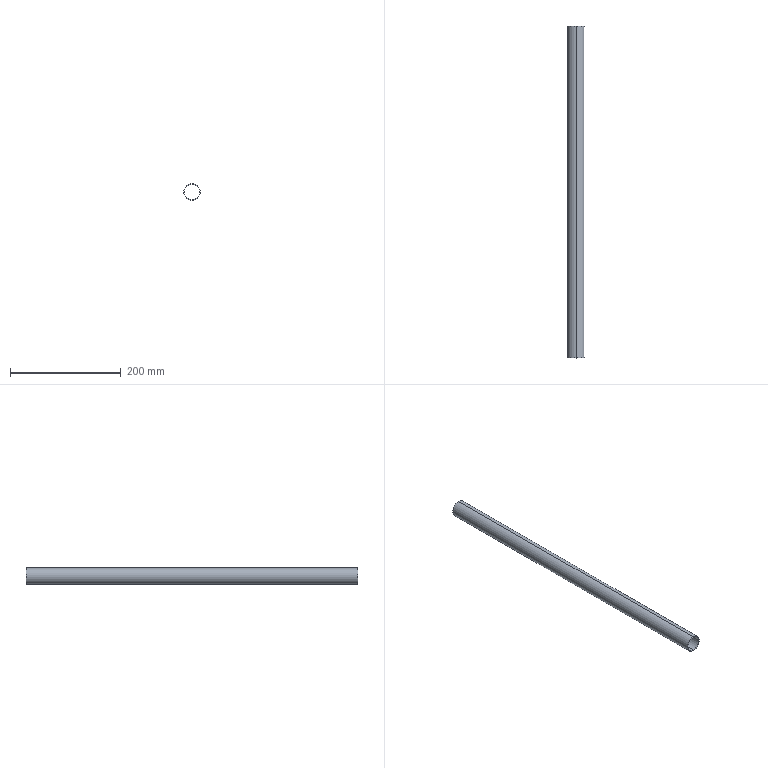Part | SolidWorks | features Sweep 1 | 1 solid | 6 faces | box 30 x 600 x 30 mm | volume 54664 mm3 | cylinder 4 | plane 2 | commonest cylinder face diameters 28 x2 30 x2
STEP:
#1=CARTESIAN_POINT('',(0.,0.,-14.));
#2=VERTEX_POINT('',#1);
#3=CARTESIAN_POINT('',(0.,0.,14.));
#4=VERTEX_POINT('',#3);
#5=CARTESIAN_POINT('',(0.,0.,0.));
#6=DIRECTION('',(0.,1.,0.));
#7=DIRECTION('',(0.,0.,1.));
#8=AXIS2_PLACEMENT_3D('',#5,#6,#7);
#9=CIRCLE('',#8,14.);
#10=EDGE_CURVE('',#2,#4,#9,.T.);
#11=ORIENTED_EDGE('',*,*,#10,.F.);
#12=CARTESIAN_POINT('',(0.,600.,-14.));
#13=VERTEX_POINT('',#12);
#14=CARTESIAN_POINT('',(0.,0.,-14.));
#15=DIRECTION('',(0.,1.,0.));
#16=VECTOR('',#15,1000.);
#17=LINE('',#14,#16);
#18=EDGE_CURVE('',#2,#13,#17,.T.);
#19=ORIENTED_EDGE('',*,*,#18,.T.);
#20=CARTESIAN_POINT('',(0.,600.,14.));
#21=VERTEX_POINT('',#20);
#22=CARTESIAN_POINT('',(0.,600.,0.));
#23=DIRECTION('',(0.,1.,0.));
#24=DIRECTION('',(0.,0.,1.));
#25=AXIS2_PLACEMENT_3D('',#22,#23,#24);
#26=CIRCLE('',#25,14.);
#27=EDGE_CURVE('',#13,#21,#26,.T.);
#28=ORIENTED_EDGE('',*,*,#27,.T.);
#29=CARTESIAN_POINT('',(0.,0.,14.));
#30=DIRECTION('',(0.,1.,0.));
#31=VECTOR('',#30,1000.);
#32=LINE('',#29,#31);
#33=EDGE_CURVE('',#4,#21,#32,.T.);
#34=ORIENTED_EDGE('',*,*,#33,.F.);
#35=EDGE_LOOP('',(#11,#19,#28,#34));
#36=FACE_OUTER_BOUND('',#35,.T.);
#37=CARTESIAN_POINT('',(0.,0.,0.));
#38=DIRECTION('',(0.,1.,0.));
#39=DIRECTION('',(0.,0.,1.));
#40=AXIS2_PLACEMENT_3D('',#37,#38,#39);
#41=CYLINDRICAL_SURFACE('',#40,14.);
#42=ADVANCED_FACE('',(#36),#41,.F.);
#43=CARTESIAN_POINT('',(0.,0.,15.));
#44=VERTEX_POINT('',#43);
#45=CARTESIAN_POINT('',(0.,0.,-15.));
#46=VERTEX_POINT('',#45);
#47=CARTESIAN_POINT('',(0.,0.,0.));
#48=DIRECTION('',(0.,1.,0.));
#49=DIRECTION('',(0.,0.,1.));
#50=AXIS2_PLACEMENT_3D('',#47,#48,#49);
#51=CIRCLE('',#50,15.);
#52=EDGE_CURVE('',#44,#46,#51,.T.);
#53=ORIENTED_EDGE('',*,*,#52,.T.);
#54=CARTESIAN_POINT('',(0.,600.,-15.));
#55=VERTEX_POINT('',#54);
#56=CARTESIAN_POINT('',(0.,0.,-15.));
#57=DIRECTION('',(0.,1.,0.));
#58=VECTOR('',#57,1000.);
#59=LINE('',#56,#58);
#60=EDGE_CURVE('',#46,#55,#59,.T.);
#61=ORIENTED_EDGE('',*,*,#60,.T.);
#62=CARTESIAN_POINT('',(0.,600.,15.));
#63=VERTEX_POINT('',#62);
#64=CARTESIAN_POINT('',(0.,600.,0.));
#65=DIRECTION('',(0.,1.,0.));
#66=DIRECTION('',(0.,0.,1.));
#67=AXIS2_PLACEMENT_3D('',#64,#65,#66);
#68=CIRCLE('',#67,15.);
#69=EDGE_CURVE('',#63,#55,#68,.T.);
#70=ORIENTED_EDGE('',*,*,#69,.F.);
#71=CARTESIAN_POINT('',(0.,0.,15.));
#72=DIRECTION('',(0.,1.,0.));
#73=VECTOR('',#72,1000.);
#74=LINE('',#71,#73);
#75=EDGE_CURVE('',#44,#63,#74,.T.);
#76=ORIENTED_EDGE('',*,*,#75,.F.);
#77=EDGE_LOOP('',(#53,#61,#70,#76));
#78=FACE_OUTER_BOUND('',#77,.T.);
#79=CARTESIAN_POINT('',(0.,0.,0.));
#80=DIRECTION('',(0.,1.,0.));
#81=DIRECTION('',(0.,0.,1.));
#82=AXIS2_PLACEMENT_3D('',#79,#80,#81);
#83=CYLINDRICAL_SURFACE('',#82,15.);
#84=ADVANCED_FACE('',(#78),#83,.T.);
#85=ORIENTED_EDGE('',*,*,#60,.F.);
#86=CARTESIAN_POINT('',(0.,0.,0.));
#87=DIRECTION('',(0.,1.,0.));
#88=DIRECTION('',(0.,0.,1.));
#89=AXIS2_PLACEMENT_3D('',#86,#87,#88);
#90=CIRCLE('',#89,15.);
#91=EDGE_CURVE('',#46,#44,#90,.T.);
#92=ORIENTED_EDGE('',*,*,#91,.T.);
#93=ORIENTED_EDGE('',*,*,#75,.T.);
#94=CARTESIAN_POINT('',(0.,600.,0.));
#95=DIRECTION('',(0.,1.,0.));
#96=DIRECTION('',(0.,0.,1.));
#97=AXIS2_PLACEMENT_3D('',#94,#95,#96);
#98=CIRCLE('',#97,15.);
#99=EDGE_CURVE('',#55,#63,#98,.T.);
#100=ORIENTED_EDGE('',*,*,#99,.F.);
#101=EDGE_LOOP('',(#85,#92,#93,#100));
#102=FACE_OUTER_BOUND('',#101,.T.);
#103=CARTESIAN_POINT('',(0.,0.,0.));
#104=DIRECTION('',(0.,1.,0.));
#105=DIRECTION('',(0.,0.,1.));
#106=AXIS2_PLACEMENT_3D('',#103,#104,#105);
#107=CYLINDRICAL_SURFACE('',#106,15.);
#108=ADVANCED_FACE('',(#102),#107,.T.);
#109=CARTESIAN_POINT('',(0.,600.,0.));
#110=DIRECTION('',(0.,1.,0.));
#111=DIRECTION('',(0.,0.,1.));
#112=AXIS2_PLACEMENT_3D('',#109,#110,#111);
#113=CIRCLE('',#112,14.);
#114=EDGE_CURVE('',#21,#13,#113,.T.);
#115=ORIENTED_EDGE('',*,*,#114,.F.);
#116=ORIENTED_EDGE('',*,*,#27,.F.);
#117=EDGE_LOOP('',(#115,#116));
#118=FACE_BOUND('',#117,.T.);
#119=ORIENTED_EDGE('',*,*,#69,.T.);
#120=ORIENTED_EDGE('',*,*,#99,.T.);
#121=EDGE_LOOP('',(#119,#120));
#122=FACE_OUTER_BOUND('',#121,.T.);
#123=CARTESIAN_POINT('',(0.,600.,0.));
#124=DIRECTION('',(0.,1.,0.));
#125=DIRECTION('',(0.,0.,1.));
#126=AXIS2_PLACEMENT_3D('',#123,#124,#125);
#127=PLANE('',#126);
#128=ADVANCED_FACE('',(#118,#122),#127,.T.);
#129=CARTESIAN_POINT('',(0.,0.,0.));
#130=DIRECTION('',(0.,1.,0.));
#131=DIRECTION('',(0.,0.,1.));
#132=AXIS2_PLACEMENT_3D('',#129,#130,#131);
#133=CIRCLE('',#132,14.);
#134=EDGE_CURVE('',#4,#2,#133,.T.);
#135=ORIENTED_EDGE('',*,*,#134,.T.);
#136=ORIENTED_EDGE('',*,*,#10,.T.);
#137=EDGE_LOOP('',(#135,#136));
#138=FACE_BOUND('',#137,.T.);
#139=ORIENTED_EDGE('',*,*,#52,.F.);
#140=ORIENTED_EDGE('',*,*,#91,.F.);
#141=EDGE_LOOP('',(#139,#140));
#142=FACE_OUTER_BOUND('',#141,.T.);
#143=CARTESIAN_POINT('',(0.,0.,0.));
#144=DIRECTION('',(0.,1.,0.));
#145=DIRECTION('',(0.,0.,1.));
#146=AXIS2_PLACEMENT_3D('',#143,#144,#145);
#147=PLANE('',#146);
#148=ADVANCED_FACE('',(#138,#142),#147,.F.);
#149=ORIENTED_EDGE('',*,*,#18,.F.);
#150=ORIENTED_EDGE('',*,*,#134,.F.);
#151=ORIENTED_EDGE('',*,*,#33,.T.);
#152=ORIENTED_EDGE('',*,*,#114,.T.);
#153=EDGE_LOOP('',(#149,#150,#151,#152));
#154=FACE_OUTER_BOUND('',#153,.T.);
#155=CARTESIAN_POINT('',(0.,0.,0.));
#156=DIRECTION('',(0.,1.,0.));
#157=DIRECTION('',(0.,0.,1.));
#158=AXIS2_PLACEMENT_3D('',#155,#156,#157);
#159=CYLINDRICAL_SURFACE('',#158,14.);
#160=ADVANCED_FACE('',(#154),#159,.F.);
#161=CLOSED_SHELL('',(#42,#84,#108,#128,#148,#160));
#162=MANIFOLD_SOLID_BREP('',#161);
#163=CARTESIAN_POINT('',(0.,0.,0.));
#164=DIRECTION('',(0.,0.,1.));
#165=DIRECTION('',(1.,0.,0.));
#166=AXIS2_PLACEMENT_3D('',#163,#164,#165);
#167=(LENGTH_UNIT()NAMED_UNIT(*)SI_UNIT(.MILLI.,.METRE.));
#168=UNCERTAINTY_MEASURE_WITH_UNIT(LENGTH_MEASURE(0.00001),#167,'','');
#169=(NAMED_UNIT(*)PLANE_ANGLE_UNIT()SI_UNIT($,.RADIAN.));
#170=(NAMED_UNIT(*)SI_UNIT($,.STERADIAN.)SOLID_ANGLE_UNIT());
#171=(GEOMETRIC_REPRESENTATION_CONTEXT(3)GLOBAL_UNCERTAINTY_ASSIGNED_CONTEXT((#168))GLOBAL_UNIT_ASSIGNED_CONTEXT((#167,#169,#170))REPRESENTATION_CONTEXT('',''));
#172=ADVANCED_BREP_SHAPE_REPRESENTATION('',(#162,#166),#171);